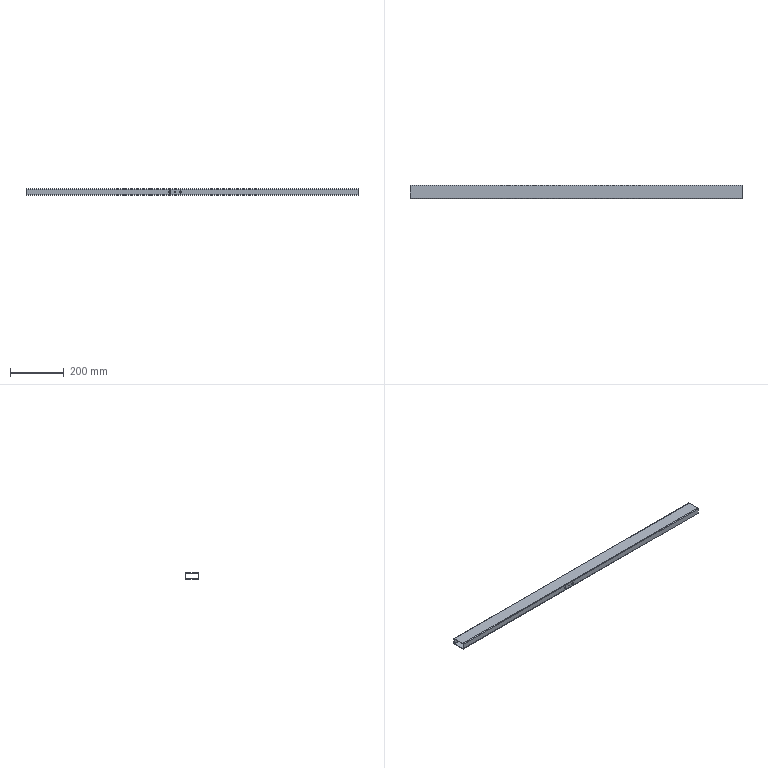Part | STEP file | 6150510 | 1 solid | 21 faces | box 1235 x 50 x 25 mm | volume 262357 mm3 | cylinder 11 | plane 10 | commonest cylinder face diameters 3 x4 5 x4 8 x2 3.2 x1
STEP:
#1=CARTESIAN_POINT('',(-617.5,-23.5,9.5));
#2=VERTEX_POINT('',#1);
#3=CARTESIAN_POINT('',(-617.5,-23.5,-9.5));
#4=VERTEX_POINT('',#3);
#5=CARTESIAN_POINT('',(-617.5,-23.5,9.5));
#6=DIRECTION('',(0.,0.,-1.));
#7=VECTOR('',#6,1000.);
#8=LINE('',#5,#7);
#9=EDGE_CURVE('',#2,#4,#8,.T.);
#10=ORIENTED_EDGE('',*,*,#9,.T.);
#11=CARTESIAN_POINT('',(-617.5,-22.,-11.));
#12=VERTEX_POINT('',#11);
#13=CARTESIAN_POINT('',(-617.5,-22.,-9.5));
#14=DIRECTION('',(1.,0.,0.));
#15=DIRECTION('',(0.,0.,-1.));
#16=AXIS2_PLACEMENT_3D('',#13,#14,#15);
#17=CIRCLE('',#16,1.5);
#18=EDGE_CURVE('',#4,#12,#17,.T.);
#19=ORIENTED_EDGE('',*,*,#18,.T.);
#20=CARTESIAN_POINT('',(-617.5,22.,-11.));
#21=VERTEX_POINT('',#20);
#22=CARTESIAN_POINT('',(-617.5,22.,-11.));
#23=DIRECTION('',(0.,1.,0.));
#24=VECTOR('',#23,1000.);
#25=LINE('',#22,#24);
#26=EDGE_CURVE('',#12,#21,#25,.T.);
#27=ORIENTED_EDGE('',*,*,#26,.T.);
#28=CARTESIAN_POINT('',(-617.5,23.5,-9.5));
#29=VERTEX_POINT('',#28);
#30=CARTESIAN_POINT('',(-617.5,22.,-9.5));
#31=DIRECTION('',(1.,0.,0.));
#32=DIRECTION('',(0.,0.,1.));
#33=AXIS2_PLACEMENT_3D('',#30,#31,#32);
#34=CIRCLE('',#33,1.5);
#35=EDGE_CURVE('',#21,#29,#34,.T.);
#36=ORIENTED_EDGE('',*,*,#35,.T.);
#37=CARTESIAN_POINT('',(-617.5,23.5,9.5));
#38=VERTEX_POINT('',#37);
#39=CARTESIAN_POINT('',(-617.5,23.5,9.5));
#40=DIRECTION('',(0.,0.,1.));
#41=VECTOR('',#40,1000.);
#42=LINE('',#39,#41);
#43=EDGE_CURVE('',#29,#38,#42,.T.);
#44=ORIENTED_EDGE('',*,*,#43,.T.);
#45=CARTESIAN_POINT('',(-617.5,22.,11.));
#46=VERTEX_POINT('',#45);
#47=CARTESIAN_POINT('',(-617.5,22.,9.5));
#48=DIRECTION('',(1.,0.,0.));
#49=DIRECTION('',(0.,0.,-1.));
#50=AXIS2_PLACEMENT_3D('',#47,#48,#49);
#51=CIRCLE('',#50,1.5);
#52=EDGE_CURVE('',#38,#46,#51,.T.);
#53=ORIENTED_EDGE('',*,*,#52,.T.);
#54=CARTESIAN_POINT('',(-617.5,-22.,11.));
#55=VERTEX_POINT('',#54);
#56=CARTESIAN_POINT('',(-617.5,22.,11.));
#57=DIRECTION('',(0.,-1.,0.));
#58=VECTOR('',#57,1000.);
#59=LINE('',#56,#58);
#60=EDGE_CURVE('',#46,#55,#59,.T.);
#61=ORIENTED_EDGE('',*,*,#60,.T.);
#62=CARTESIAN_POINT('',(-617.5,-22.,9.5));
#63=DIRECTION('',(1.,0.,0.));
#64=DIRECTION('',(0.,0.,-1.));
#65=AXIS2_PLACEMENT_3D('',#62,#63,#64);
#66=CIRCLE('',#65,1.5);
#67=EDGE_CURVE('',#55,#2,#66,.T.);
#68=ORIENTED_EDGE('',*,*,#67,.T.);
#69=EDGE_LOOP('',(#10,#19,#27,#36,#44,#53,#61,#68));
#70=FACE_BOUND('',#69,.T.);
#71=CARTESIAN_POINT('',(-617.5,-25.,10.));
#72=VERTEX_POINT('',#71);
#73=CARTESIAN_POINT('',(-617.5,-25.,-10.));
#74=VERTEX_POINT('',#73);
#75=CARTESIAN_POINT('',(-617.5,-25.,12.5));
#76=DIRECTION('',(0.,0.,-1.));
#77=VECTOR('',#76,1000.);
#78=LINE('',#75,#77);
#79=EDGE_CURVE('',#72,#74,#78,.T.);
#80=ORIENTED_EDGE('',*,*,#79,.F.);
#81=CARTESIAN_POINT('',(-617.5,-22.5,12.5));
#82=VERTEX_POINT('',#81);
#83=CARTESIAN_POINT('',(-617.5,-22.5,10.));
#84=DIRECTION('',(-1.,0.,0.));
#85=DIRECTION('',(0.,0.,-1.));
#86=AXIS2_PLACEMENT_3D('',#83,#84,#85);
#87=CIRCLE('',#86,2.5);
#88=EDGE_CURVE('',#72,#82,#87,.T.);
#89=ORIENTED_EDGE('',*,*,#88,.T.);
#90=CARTESIAN_POINT('',(-617.5,22.5,12.5));
#91=VERTEX_POINT('',#90);
#92=CARTESIAN_POINT('',(-617.5,25.,12.5));
#93=DIRECTION('',(0.,-1.,0.));
#94=VECTOR('',#93,1000.);
#95=LINE('',#92,#94);
#96=EDGE_CURVE('',#91,#82,#95,.T.);
#97=ORIENTED_EDGE('',*,*,#96,.F.);
#98=CARTESIAN_POINT('',(-617.5,25.,10.));
#99=VERTEX_POINT('',#98);
#100=CARTESIAN_POINT('',(-617.5,22.5,10.));
#101=DIRECTION('',(-1.,0.,0.));
#102=DIRECTION('',(0.,0.,-1.));
#103=AXIS2_PLACEMENT_3D('',#100,#101,#102);
#104=CIRCLE('',#103,2.5);
#105=EDGE_CURVE('',#91,#99,#104,.T.);
#106=ORIENTED_EDGE('',*,*,#105,.T.);
#107=CARTESIAN_POINT('',(-617.5,25.,-10.));
#108=VERTEX_POINT('',#107);
#109=CARTESIAN_POINT('',(-617.5,25.,12.5));
#110=DIRECTION('',(0.,0.,-1.));
#111=VECTOR('',#110,1000.);
#112=LINE('',#109,#111);
#113=EDGE_CURVE('',#99,#108,#112,.T.);
#114=ORIENTED_EDGE('',*,*,#113,.T.);
#115=CARTESIAN_POINT('',(-617.5,22.5,-12.5));
#116=VERTEX_POINT('',#115);
#117=CARTESIAN_POINT('',(-617.5,22.5,-10.));
#118=DIRECTION('',(-1.,0.,0.));
#119=DIRECTION('',(0.,0.,-1.));
#120=AXIS2_PLACEMENT_3D('',#117,#118,#119);
#121=CIRCLE('',#120,2.5);
#122=EDGE_CURVE('',#108,#116,#121,.T.);
#123=ORIENTED_EDGE('',*,*,#122,.T.);
#124=CARTESIAN_POINT('',(-617.5,-22.5,-12.5));
#125=VERTEX_POINT('',#124);
#126=CARTESIAN_POINT('',(-617.5,25.,-12.5));
#127=DIRECTION('',(0.,-1.,0.));
#128=VECTOR('',#127,1000.);
#129=LINE('',#126,#128);
#130=EDGE_CURVE('',#116,#125,#129,.T.);
#131=ORIENTED_EDGE('',*,*,#130,.T.);
#132=CARTESIAN_POINT('',(-617.5,-22.5,-10.));
#133=DIRECTION('',(-1.,0.,0.));
#134=DIRECTION('',(0.,0.,-1.));
#135=AXIS2_PLACEMENT_3D('',#132,#133,#134);
#136=CIRCLE('',#135,2.5);
#137=EDGE_CURVE('',#125,#74,#136,.T.);
#138=ORIENTED_EDGE('',*,*,#137,.T.);
#139=EDGE_LOOP('',(#80,#89,#97,#106,#114,#123,#131,#138));
#140=FACE_OUTER_BOUND('',#139,.T.);
#141=CARTESIAN_POINT('',(-617.5,25.,12.5));
#142=DIRECTION('',(1.,0.,0.));
#143=DIRECTION('',(0.,0.,-1.));
#144=AXIS2_PLACEMENT_3D('',#141,#142,#143);
#145=PLANE('',#144);
#146=ADVANCED_FACE('',(#70,#140),#145,.F.);
#147=CARTESIAN_POINT('',(-78.5,-25.,0.));
#148=VERTEX_POINT('',#147);
#149=CARTESIAN_POINT('',(-82.5,-25.,0.));
#150=DIRECTION('',(0.,-1.,0.));
#151=DIRECTION('',(1.,0.,0.));
#152=AXIS2_PLACEMENT_3D('',#149,#150,#151);
#153=CIRCLE('',#152,4.);
#154=EDGE_CURVE('',#148,#148,#153,.T.);
#155=ORIENTED_EDGE('',*,*,#154,.F.);
#156=EDGE_LOOP('',(#155));
#157=FACE_BOUND('',#156,.T.);
#158=CARTESIAN_POINT('',(-38.5,-25.,0.));
#159=VERTEX_POINT('',#158);
#160=CARTESIAN_POINT('',(-42.5,-25.,0.));
#161=DIRECTION('',(0.,-1.,0.));
#162=DIRECTION('',(1.,0.,0.));
#163=AXIS2_PLACEMENT_3D('',#160,#161,#162);
#164=CIRCLE('',#163,4.);
#165=EDGE_CURVE('',#159,#159,#164,.T.);
#166=ORIENTED_EDGE('',*,*,#165,.F.);
#167=EDGE_LOOP('',(#166));
#168=FACE_BOUND('',#167,.T.);
#169=CARTESIAN_POINT('',(-60.9,-25.,0.));
#170=VERTEX_POINT('',#169);
#171=CARTESIAN_POINT('',(-62.5,-25.,0.));
#172=DIRECTION('',(0.,-1.,0.));
#173=DIRECTION('',(1.,0.,0.));
#174=AXIS2_PLACEMENT_3D('',#171,#172,#173);
#175=CIRCLE('',#174,1.6);
#176=EDGE_CURVE('',#170,#170,#175,.T.);
#177=ORIENTED_EDGE('',*,*,#176,.F.);
#178=EDGE_LOOP('',(#177));
#179=FACE_BOUND('',#178,.T.);
#180=CARTESIAN_POINT('',(617.5,-25.,10.));
#181=VERTEX_POINT('',#180);
#182=CARTESIAN_POINT('',(617.5,-25.,-10.));
#183=VERTEX_POINT('',#182);
#184=CARTESIAN_POINT('',(617.5,-25.,12.5));
#185=DIRECTION('',(0.,0.,-1.));
#186=VECTOR('',#185,1000.);
#187=LINE('',#184,#186);
#188=EDGE_CURVE('',#181,#183,#187,.T.);
#189=ORIENTED_EDGE('',*,*,#188,.F.);
#190=CARTESIAN_POINT('',(-617.5,-25.,10.));
#191=DIRECTION('',(-1.,0.,0.));
#192=VECTOR('',#191,1000.);
#193=LINE('',#190,#192);
#194=EDGE_CURVE('',#181,#72,#193,.T.);
#195=ORIENTED_EDGE('',*,*,#194,.T.);
#196=ORIENTED_EDGE('',*,*,#79,.T.);
#197=CARTESIAN_POINT('',(-617.5,-25.,-10.));
#198=DIRECTION('',(1.,0.,0.));
#199=VECTOR('',#198,1000.);
#200=LINE('',#197,#199);
#201=EDGE_CURVE('',#74,#183,#200,.T.);
#202=ORIENTED_EDGE('',*,*,#201,.T.);
#203=EDGE_LOOP('',(#189,#195,#196,#202));
#204=FACE_OUTER_BOUND('',#203,.T.);
#205=CARTESIAN_POINT('',(-617.5,-25.,12.5));
#206=DIRECTION('',(0.,1.,0.));
#207=DIRECTION('',(-1.,0.,0.));
#208=AXIS2_PLACEMENT_3D('',#205,#206,#207);
#209=PLANE('',#208);
#210=ADVANCED_FACE('',(#157,#168,#179,#204),#209,.F.);
#211=CARTESIAN_POINT('',(617.5,-22.,-11.));
#212=VERTEX_POINT('',#211);
#213=CARTESIAN_POINT('',(617.5,22.,-11.));
#214=VERTEX_POINT('',#213);
#215=CARTESIAN_POINT('',(617.5,22.,-11.));
#216=DIRECTION('',(0.,1.,0.));
#217=VECTOR('',#216,1000.);
#218=LINE('',#215,#217);
#219=EDGE_CURVE('',#212,#214,#218,.T.);
#220=ORIENTED_EDGE('',*,*,#219,.F.);
#221=CARTESIAN_POINT('',(617.5,-23.5,-9.5));
#222=VERTEX_POINT('',#221);
#223=CARTESIAN_POINT('',(617.5,-22.,-9.5));
#224=DIRECTION('',(1.,0.,0.));
#225=DIRECTION('',(0.,0.,-1.));
#226=AXIS2_PLACEMENT_3D('',#223,#224,#225);
#227=CIRCLE('',#226,1.5);
#228=EDGE_CURVE('',#222,#212,#227,.T.);
#229=ORIENTED_EDGE('',*,*,#228,.F.);
#230=CARTESIAN_POINT('',(617.5,-23.5,9.5));
#231=VERTEX_POINT('',#230);
#232=CARTESIAN_POINT('',(617.5,-23.5,9.5));
#233=DIRECTION('',(0.,0.,-1.));
#234=VECTOR('',#233,1000.);
#235=LINE('',#232,#234);
#236=EDGE_CURVE('',#231,#222,#235,.T.);
#237=ORIENTED_EDGE('',*,*,#236,.F.);
#238=CARTESIAN_POINT('',(617.5,-22.,11.));
#239=VERTEX_POINT('',#238);
#240=CARTESIAN_POINT('',(617.5,-22.,9.5));
#241=DIRECTION('',(1.,0.,0.));
#242=DIRECTION('',(0.,0.,-1.));
#243=AXIS2_PLACEMENT_3D('',#240,#241,#242);
#244=CIRCLE('',#243,1.5);
#245=EDGE_CURVE('',#239,#231,#244,.T.);
#246=ORIENTED_EDGE('',*,*,#245,.F.);
#247=CARTESIAN_POINT('',(617.5,22.,11.));
#248=VERTEX_POINT('',#247);
#249=CARTESIAN_POINT('',(617.5,22.,11.));
#250=DIRECTION('',(0.,-1.,0.));
#251=VECTOR('',#250,1000.);
#252=LINE('',#249,#251);
#253=EDGE_CURVE('',#248,#239,#252,.T.);
#254=ORIENTED_EDGE('',*,*,#253,.F.);
#255=CARTESIAN_POINT('',(617.5,23.5,9.5));
#256=VERTEX_POINT('',#255);
#257=CARTESIAN_POINT('',(617.5,22.,9.5));
#258=DIRECTION('',(1.,0.,0.));
#259=DIRECTION('',(0.,0.,-1.));
#260=AXIS2_PLACEMENT_3D('',#257,#258,#259);
#261=CIRCLE('',#260,1.5);
#262=EDGE_CURVE('',#256,#248,#261,.T.);
#263=ORIENTED_EDGE('',*,*,#262,.F.);
#264=CARTESIAN_POINT('',(617.5,23.5,-9.5));
#265=VERTEX_POINT('',#264);
#266=CARTESIAN_POINT('',(617.5,23.5,9.5));
#267=DIRECTION('',(0.,0.,1.));
#268=VECTOR('',#267,1000.);
#269=LINE('',#266,#268);
#270=EDGE_CURVE('',#265,#256,#269,.T.);
#271=ORIENTED_EDGE('',*,*,#270,.F.);
#272=CARTESIAN_POINT('',(617.5,22.,-9.5));
#273=DIRECTION('',(1.,0.,0.));
#274=DIRECTION('',(0.,0.,1.));
#275=AXIS2_PLACEMENT_3D('',#272,#273,#274);
#276=CIRCLE('',#275,1.5);
#277=EDGE_CURVE('',#214,#265,#276,.T.);
#278=ORIENTED_EDGE('',*,*,#277,.F.);
#279=EDGE_LOOP('',(#220,#229,#237,#246,#254,#263,#271,#278));
#280=FACE_BOUND('',#279,.T.);
#281=CARTESIAN_POINT('',(617.5,-22.5,12.5));
#282=VERTEX_POINT('',#281);
#283=CARTESIAN_POINT('',(617.5,22.5,12.5));
#284=VERTEX_POINT('',#283);
#285=CARTESIAN_POINT('',(617.5,25.,12.5));
#286=DIRECTION('',(0.,1.,0.));
#287=VECTOR('',#286,1000.);
#288=LINE('',#285,#287);
#289=EDGE_CURVE('',#282,#284,#288,.T.);
#290=ORIENTED_EDGE('',*,*,#289,.F.);
#291=CARTESIAN_POINT('',(617.5,-22.5,10.));
#292=DIRECTION('',(1.,0.,0.));
#293=DIRECTION('',(0.,0.,1.));
#294=AXIS2_PLACEMENT_3D('',#291,#292,#293);
#295=CIRCLE('',#294,2.5);
#296=EDGE_CURVE('',#282,#181,#295,.T.);
#297=ORIENTED_EDGE('',*,*,#296,.T.);
#298=ORIENTED_EDGE('',*,*,#188,.T.);
#299=CARTESIAN_POINT('',(617.5,-22.5,-12.5));
#300=VERTEX_POINT('',#299);
#301=CARTESIAN_POINT('',(617.5,-22.5,-10.));
#302=DIRECTION('',(1.,0.,0.));
#303=DIRECTION('',(0.,0.,1.));
#304=AXIS2_PLACEMENT_3D('',#301,#302,#303);
#305=CIRCLE('',#304,2.5);
#306=EDGE_CURVE('',#183,#300,#305,.T.);
#307=ORIENTED_EDGE('',*,*,#306,.T.);
#308=CARTESIAN_POINT('',(617.5,22.5,-12.5));
#309=VERTEX_POINT('',#308);
#310=CARTESIAN_POINT('',(617.5,25.,-12.5));
#311=DIRECTION('',(0.,1.,0.));
#312=VECTOR('',#311,1000.);
#313=LINE('',#310,#312);
#314=EDGE_CURVE('',#300,#309,#313,.T.);
#315=ORIENTED_EDGE('',*,*,#314,.T.);
#316=CARTESIAN_POINT('',(617.5,25.,-10.));
#317=VERTEX_POINT('',#316);
#318=CARTESIAN_POINT('',(617.5,22.5,-10.));
#319=DIRECTION('',(1.,0.,0.));
#320=DIRECTION('',(0.,0.,1.));
#321=AXIS2_PLACEMENT_3D('',#318,#319,#320);
#322=CIRCLE('',#321,2.5);
#323=EDGE_CURVE('',#309,#317,#322,.T.);
#324=ORIENTED_EDGE('',*,*,#323,.T.);
#325=CARTESIAN_POINT('',(617.5,25.,10.));
#326=VERTEX_POINT('',#325);
#327=CARTESIAN_POINT('',(617.5,25.,12.5));
#328=DIRECTION('',(0.,0.,-1.));
#329=VECTOR('',#328,1000.);
#330=LINE('',#327,#329);
#331=EDGE_CURVE('',#326,#317,#330,.T.);
#332=ORIENTED_EDGE('',*,*,#331,.F.);
#333=CARTESIAN_POINT('',(617.5,22.5,10.));
#334=DIRECTION('',(1.,0.,0.));
#335=DIRECTION('',(0.,0.,1.));
#336=AXIS2_PLACEMENT_3D('',#333,#334,#335);
#337=CIRCLE('',#336,2.5);
#338=EDGE_CURVE('',#326,#284,#337,.T.);
#339=ORIENTED_EDGE('',*,*,#338,.T.);
#340=EDGE_LOOP('',(#290,#297,#298,#307,#315,#324,#332,#339));
#341=FACE_OUTER_BOUND('',#340,.T.);
#342=CARTESIAN_POINT('',(617.5,25.,12.5));
#343=DIRECTION('',(-1.,0.,0.));
#344=DIRECTION('',(0.,0.,1.));
#345=AXIS2_PLACEMENT_3D('',#342,#343,#344);
#346=PLANE('',#345);
#347=ADVANCED_FACE('',(#280,#341),#346,.F.);
#348=ORIENTED_EDGE('',*,*,#331,.T.);
#349=CARTESIAN_POINT('',(-617.5,25.,-10.));
#350=DIRECTION('',(-1.,0.,0.));
#351=VECTOR('',#350,1000.);
#352=LINE('',#349,#351);
#353=EDGE_CURVE('',#317,#108,#352,.T.);
#354=ORIENTED_EDGE('',*,*,#353,.T.);
#355=ORIENTED_EDGE('',*,*,#113,.F.);
#356=CARTESIAN_POINT('',(617.5,25.,10.));
#357=DIRECTION('',(1.,0.,0.));
#358=VECTOR('',#357,1000.);
#359=LINE('',#356,#358);
#360=EDGE_CURVE('',#99,#326,#359,.T.);
#361=ORIENTED_EDGE('',*,*,#360,.T.);
#362=EDGE_LOOP('',(#348,#354,#355,#361));
#363=FACE_OUTER_BOUND('',#362,.T.);
#364=CARTESIAN_POINT('',(-617.5,25.,12.5));
#365=DIRECTION('',(0.,-1.,0.));
#366=DIRECTION('',(0.,0.,-1.));
#367=AXIS2_PLACEMENT_3D('',#364,#365,#366);
#368=PLANE('',#367);
#369=ADVANCED_FACE('',(#363),#368,.F.);
#370=ORIENTED_EDGE('',*,*,#96,.T.);
#371=CARTESIAN_POINT('',(617.5,-22.5,12.5));
#372=DIRECTION('',(1.,0.,0.));
#373=VECTOR('',#372,1000.);
#374=LINE('',#371,#373);
#375=EDGE_CURVE('',#82,#282,#374,.T.);
#376=ORIENTED_EDGE('',*,*,#375,.T.);
#377=ORIENTED_EDGE('',*,*,#289,.T.);
#378=CARTESIAN_POINT('',(-617.5,22.5,12.5));
#379=DIRECTION('',(-1.,0.,0.));
#380=VECTOR('',#379,1000.);
#381=LINE('',#378,#380);
#382=EDGE_CURVE('',#284,#91,#381,.T.);
#383=ORIENTED_EDGE('',*,*,#382,.T.);
#384=EDGE_LOOP('',(#370,#376,#377,#383));
#385=FACE_OUTER_BOUND('',#384,.T.);
#386=CARTESIAN_POINT('',(-617.5,25.,12.5));
#387=DIRECTION('',(0.,0.,1.));
#388=DIRECTION('',(1.,0.,0.));
#389=AXIS2_PLACEMENT_3D('',#386,#387,#388);
#390=PLANE('',#389);
#391=ADVANCED_FACE('',(#385),#390,.T.);
#392=ORIENTED_EDGE('',*,*,#314,.F.);
#393=CARTESIAN_POINT('',(-617.5,-22.5,-12.5));
#394=DIRECTION('',(-1.,0.,0.));
#395=VECTOR('',#394,1000.);
#396=LINE('',#393,#395);
#397=EDGE_CURVE('',#300,#125,#396,.T.);
#398=ORIENTED_EDGE('',*,*,#397,.T.);
#399=ORIENTED_EDGE('',*,*,#130,.F.);
#400=CARTESIAN_POINT('',(-617.5,22.5,-12.5));
#401=DIRECTION('',(1.,0.,0.));
#402=VECTOR('',#401,1000.);
#403=LINE('',#400,#402);
#404=EDGE_CURVE('',#116,#309,#403,.T.);
#405=ORIENTED_EDGE('',*,*,#404,.T.);
#406=EDGE_LOOP('',(#392,#398,#399,#405));
#407=FACE_OUTER_BOUND('',#406,.T.);
#408=CARTESIAN_POINT('',(-617.5,25.,-12.5));
#409=DIRECTION('',(0.,0.,1.));
#410=DIRECTION('',(1.,0.,0.));
#411=AXIS2_PLACEMENT_3D('',#408,#409,#410);
#412=PLANE('',#411);
#413=ADVANCED_FACE('',(#407),#412,.F.);
#414=ORIENTED_EDGE('',*,*,#88,.F.);
#415=ORIENTED_EDGE('',*,*,#194,.F.);
#416=ORIENTED_EDGE('',*,*,#296,.F.);
#417=ORIENTED_EDGE('',*,*,#375,.F.);
#418=EDGE_LOOP('',(#414,#415,#416,#417));
#419=FACE_OUTER_BOUND('',#418,.T.);
#420=CARTESIAN_POINT('',(-617.5,-22.5,10.));
#421=DIRECTION('',(-1.,0.,0.));
#422=DIRECTION('',(0.,-1.,0.));
#423=AXIS2_PLACEMENT_3D('',#420,#421,#422);
#424=CYLINDRICAL_SURFACE('',#423,2.5);
#425=ADVANCED_FACE('',(#419),#424,.T.);
#426=ORIENTED_EDGE('',*,*,#137,.F.);
#427=ORIENTED_EDGE('',*,*,#397,.F.);
#428=ORIENTED_EDGE('',*,*,#306,.F.);
#429=ORIENTED_EDGE('',*,*,#201,.F.);
#430=EDGE_LOOP('',(#426,#427,#428,#429));
#431=FACE_OUTER_BOUND('',#430,.T.);
#432=CARTESIAN_POINT('',(-617.5,-22.5,-10.));
#433=DIRECTION('',(1.,0.,0.));
#434=DIRECTION('',(0.,1.,0.));
#435=AXIS2_PLACEMENT_3D('',#432,#433,#434);
#436=CYLINDRICAL_SURFACE('',#435,2.5);
#437=ADVANCED_FACE('',(#431),#436,.T.);
#438=ORIENTED_EDGE('',*,*,#323,.F.);
#439=ORIENTED_EDGE('',*,*,#404,.F.);
#440=ORIENTED_EDGE('',*,*,#122,.F.);
#441=ORIENTED_EDGE('',*,*,#353,.F.);
#442=EDGE_LOOP('',(#438,#439,#440,#441));
#443=FACE_OUTER_BOUND('',#442,.T.);
#444=CARTESIAN_POINT('',(-617.5,22.5,-10.));
#445=DIRECTION('',(-1.,0.,0.));
#446=DIRECTION('',(0.,0.,1.));
#447=AXIS2_PLACEMENT_3D('',#444,#445,#446);
#448=CYLINDRICAL_SURFACE('',#447,2.5);
#449=ADVANCED_FACE('',(#443),#448,.T.);
#450=ORIENTED_EDGE('',*,*,#338,.F.);
#451=ORIENTED_EDGE('',*,*,#360,.F.);
#452=ORIENTED_EDGE('',*,*,#105,.F.);
#453=ORIENTED_EDGE('',*,*,#382,.F.);
#454=EDGE_LOOP('',(#450,#451,#452,#453));
#455=FACE_OUTER_BOUND('',#454,.T.);
#456=CARTESIAN_POINT('',(-617.5,22.5,10.));
#457=DIRECTION('',(1.,0.,0.));
#458=DIRECTION('',(0.,0.,-1.));
#459=AXIS2_PLACEMENT_3D('',#456,#457,#458);
#460=CYLINDRICAL_SURFACE('',#459,2.5);
#461=ADVANCED_FACE('',(#455),#460,.T.);
#462=ORIENTED_EDGE('',*,*,#228,.T.);
#463=CARTESIAN_POINT('',(-617.5,-22.,-11.));
#464=DIRECTION('',(1.,0.,0.));
#465=VECTOR('',#464,1000.);
#466=LINE('',#463,#465);
#467=EDGE_CURVE('',#12,#212,#466,.T.);
#468=ORIENTED_EDGE('',*,*,#467,.F.);
#469=ORIENTED_EDGE('',*,*,#18,.F.);
#470=CARTESIAN_POINT('',(-617.5,-23.5,-9.5));
#471=DIRECTION('',(1.,0.,0.));
#472=VECTOR('',#471,1000.);
#473=LINE('',#470,#472);
#474=EDGE_CURVE('',#4,#222,#473,.T.);
#475=ORIENTED_EDGE('',*,*,#474,.T.);
#476=EDGE_LOOP('',(#462,#468,#469,#475));
#477=FACE_OUTER_BOUND('',#476,.T.);
#478=CARTESIAN_POINT('',(-617.5,-22.,-9.5));
#479=DIRECTION('',(1.,0.,0.));
#480=DIRECTION('',(0.,0.,-1.));
#481=AXIS2_PLACEMENT_3D('',#478,#479,#480);
#482=CYLINDRICAL_SURFACE('',#481,1.5);
#483=ADVANCED_FACE('',(#477),#482,.F.);
#484=CARTESIAN_POINT('',(-82.5,-23.5,-4.));
#485=VERTEX_POINT('',#484);
#486=CARTESIAN_POINT('',(-82.5,-23.5,0.));
#487=DIRECTION('',(0.,-1.,0.));
#488=DIRECTION('',(0.,0.,-1.));
#489=AXIS2_PLACEMENT_3D('',#486,#487,#488);
#490=CIRCLE('',#489,4.);
#491=EDGE_CURVE('',#485,#485,#490,.T.);
#492=ORIENTED_EDGE('',*,*,#491,.T.);
#493=EDGE_LOOP('',(#492));
#494=FACE_BOUND('',#493,.T.);
#495=CARTESIAN_POINT('',(-42.5,-23.5,-4.));
#496=VERTEX_POINT('',#495);
#497=CARTESIAN_POINT('',(-42.5,-23.5,0.));
#498=DIRECTION('',(0.,-1.,0.));
#499=DIRECTION('',(0.,0.,-1.));
#500=AXIS2_PLACEMENT_3D('',#497,#498,#499);
#501=CIRCLE('',#500,4.);
#502=EDGE_CURVE('',#496,#496,#501,.T.);
#503=ORIENTED_EDGE('',*,*,#502,.T.);
#504=EDGE_LOOP('',(#503));
#505=FACE_BOUND('',#504,.T.);
#506=CARTESIAN_POINT('',(-62.5,-23.5,-1.6));
#507=VERTEX_POINT('',#506);
#508=CARTESIAN_POINT('',(-62.5,-23.5,0.));
#509=DIRECTION('',(0.,-1.,0.));
#510=DIRECTION('',(0.,0.,-1.));
#511=AXIS2_PLACEMENT_3D('',#508,#509,#510);
#512=CIRCLE('',#511,1.6);
#513=EDGE_CURVE('',#507,#507,#512,.T.);
#514=ORIENTED_EDGE('',*,*,#513,.T.);
#515=EDGE_LOOP('',(#514));
#516=FACE_BOUND('',#515,.T.);
#517=ORIENTED_EDGE('',*,*,#236,.T.);
#518=ORIENTED_EDGE('',*,*,#474,.F.);
#519=ORIENTED_EDGE('',*,*,#9,.F.);
#520=CARTESIAN_POINT('',(-617.5,-23.5,9.5));
#521=DIRECTION('',(1.,0.,0.));
#522=VECTOR('',#521,1000.);
#523=LINE('',#520,#522);
#524=EDGE_CURVE('',#2,#231,#523,.T.);
#525=ORIENTED_EDGE('',*,*,#524,.T.);
#526=EDGE_LOOP('',(#517,#518,#519,#525));
#527=FACE_OUTER_BOUND('',#526,.T.);
#528=CARTESIAN_POINT('',(-617.5,-23.5,9.5));
#529=DIRECTION('',(0.,-1.,0.));
#530=DIRECTION('',(0.,0.,-1.));
#531=AXIS2_PLACEMENT_3D('',#528,#529,#530);
#532=PLANE('',#531);
#533=ADVANCED_FACE('',(#494,#505,#516,#527),#532,.F.);
#534=ORIENTED_EDGE('',*,*,#245,.T.);
#535=ORIENTED_EDGE('',*,*,#524,.F.);
#536=ORIENTED_EDGE('',*,*,#67,.F.);
#537=CARTESIAN_POINT('',(-617.5,-22.,11.));
#538=DIRECTION('',(1.,0.,0.));
#539=VECTOR('',#538,1000.);
#540=LINE('',#537,#539);
#541=EDGE_CURVE('',#55,#239,#540,.T.);
#542=ORIENTED_EDGE('',*,*,#541,.T.);
#543=EDGE_LOOP('',(#534,#535,#536,#542));
#544=FACE_OUTER_BOUND('',#543,.T.);
#545=CARTESIAN_POINT('',(-617.5,-22.,9.5));
#546=DIRECTION('',(1.,0.,0.));
#547=DIRECTION('',(0.,0.,-1.));
#548=AXIS2_PLACEMENT_3D('',#545,#546,#547);
#549=CYLINDRICAL_SURFACE('',#548,1.5);
#550=ADVANCED_FACE('',(#544),#549,.F.);
#551=ORIENTED_EDGE('',*,*,#253,.T.);
#552=ORIENTED_EDGE('',*,*,#541,.F.);
#553=ORIENTED_EDGE('',*,*,#60,.F.);
#554=CARTESIAN_POINT('',(-617.5,22.,11.));
#555=DIRECTION('',(1.,0.,0.));
#556=VECTOR('',#555,1000.);
#557=LINE('',#554,#556);
#558=EDGE_CURVE('',#46,#248,#557,.T.);
#559=ORIENTED_EDGE('',*,*,#558,.T.);
#560=EDGE_LOOP('',(#551,#552,#553,#559));
#561=FACE_OUTER_BOUND('',#560,.T.);
#562=CARTESIAN_POINT('',(-617.5,22.,11.));
#563=DIRECTION('',(0.,0.,1.));
#564=DIRECTION('',(0.,-1.,0.));
#565=AXIS2_PLACEMENT_3D('',#562,#563,#564);
#566=PLANE('',#565);
#567=ADVANCED_FACE('',(#561),#566,.F.);
#568=ORIENTED_EDGE('',*,*,#262,.T.);
#569=ORIENTED_EDGE('',*,*,#558,.F.);
#570=ORIENTED_EDGE('',*,*,#52,.F.);
#571=CARTESIAN_POINT('',(-617.5,23.5,9.5));
#572=DIRECTION('',(1.,0.,0.));
#573=VECTOR('',#572,1000.);
#574=LINE('',#571,#573);
#575=EDGE_CURVE('',#38,#256,#574,.T.);
#576=ORIENTED_EDGE('',*,*,#575,.T.);
#577=EDGE_LOOP('',(#568,#569,#570,#576));
#578=FACE_OUTER_BOUND('',#577,.T.);
#579=CARTESIAN_POINT('',(-617.5,22.,9.5));
#580=DIRECTION('',(1.,0.,0.));
#581=DIRECTION('',(0.,0.,-1.));
#582=AXIS2_PLACEMENT_3D('',#579,#580,#581);
#583=CYLINDRICAL_SURFACE('',#582,1.5);
#584=ADVANCED_FACE('',(#578),#583,.F.);
#585=ORIENTED_EDGE('',*,*,#270,.T.);
#586=ORIENTED_EDGE('',*,*,#575,.F.);
#587=ORIENTED_EDGE('',*,*,#43,.F.);
#588=CARTESIAN_POINT('',(-617.5,23.5,-9.5));
#589=DIRECTION('',(1.,0.,0.));
#590=VECTOR('',#589,1000.);
#591=LINE('',#588,#590);
#592=EDGE_CURVE('',#29,#265,#591,.T.);
#593=ORIENTED_EDGE('',*,*,#592,.T.);
#594=EDGE_LOOP('',(#585,#586,#587,#593));
#595=FACE_OUTER_BOUND('',#594,.T.);
#596=CARTESIAN_POINT('',(-617.5,23.5,9.5));
#597=DIRECTION('',(0.,1.,0.));
#598=DIRECTION('',(0.,0.,1.));
#599=AXIS2_PLACEMENT_3D('',#596,#597,#598);
#600=PLANE('',#599);
#601=ADVANCED_FACE('',(#595),#600,.F.);
#602=ORIENTED_EDGE('',*,*,#277,.T.);
#603=ORIENTED_EDGE('',*,*,#592,.F.);
#604=ORIENTED_EDGE('',*,*,#35,.F.);
#605=CARTESIAN_POINT('',(-617.5,22.,-11.));
#606=DIRECTION('',(1.,0.,0.));
#607=VECTOR('',#606,1000.);
#608=LINE('',#605,#607);
#609=EDGE_CURVE('',#21,#214,#608,.T.);
#610=ORIENTED_EDGE('',*,*,#609,.T.);
#611=EDGE_LOOP('',(#602,#603,#604,#610));
#612=FACE_OUTER_BOUND('',#611,.T.);
#613=CARTESIAN_POINT('',(-617.5,22.,-9.5));
#614=DIRECTION('',(1.,0.,0.));
#615=DIRECTION('',(0.,0.,-1.));
#616=AXIS2_PLACEMENT_3D('',#613,#614,#615);
#617=CYLINDRICAL_SURFACE('',#616,1.5);
#618=ADVANCED_FACE('',(#612),#617,.F.);
#619=ORIENTED_EDGE('',*,*,#219,.T.);
#620=ORIENTED_EDGE('',*,*,#609,.F.);
#621=ORIENTED_EDGE('',*,*,#26,.F.);
#622=ORIENTED_EDGE('',*,*,#467,.T.);
#623=EDGE_LOOP('',(#619,#620,#621,#622));
#624=FACE_OUTER_BOUND('',#623,.T.);
#625=CARTESIAN_POINT('',(-617.5,22.,-11.));
#626=DIRECTION('',(0.,0.,-1.));
#627=DIRECTION('',(0.,1.,0.));
#628=AXIS2_PLACEMENT_3D('',#625,#626,#627);
#629=PLANE('',#628);
#630=ADVANCED_FACE('',(#624),#629,.F.);
#631=ORIENTED_EDGE('',*,*,#176,.T.);
#632=EDGE_LOOP('',(#631));
#633=FACE_OUTER_BOUND('',#632,.T.);
#634=ORIENTED_EDGE('',*,*,#513,.F.);
#635=EDGE_LOOP('',(#634));
#636=FACE_OUTER_BOUND('',#635,.T.);
#637=CARTESIAN_POINT('',(-62.5,-15.,0.));
#638=DIRECTION('',(0.,-1.,0.));
#639=DIRECTION('',(1.,0.,0.));
#640=AXIS2_PLACEMENT_3D('',#637,#638,#639);
#641=CYLINDRICAL_SURFACE('',#640,1.6);
#642=ADVANCED_FACE('',(#633,#636),#641,.F.);
#643=ORIENTED_EDGE('',*,*,#165,.T.);
#644=EDGE_LOOP('',(#643));
#645=FACE_OUTER_BOUND('',#644,.T.);
#646=ORIENTED_EDGE('',*,*,#502,.F.);
#647=EDGE_LOOP('',(#646));
#648=FACE_OUTER_BOUND('',#647,.T.);
#649=CARTESIAN_POINT('',(-42.5,-15.,0.));
#650=DIRECTION('',(0.,-1.,0.));
#651=DIRECTION('',(1.,0.,0.));
#652=AXIS2_PLACEMENT_3D('',#649,#650,#651);
#653=CYLINDRICAL_SURFACE('',#652,4.);
#654=ADVANCED_FACE('',(#645,#648),#653,.F.);
#655=ORIENTED_EDGE('',*,*,#154,.T.);
#656=EDGE_LOOP('',(#655));
#657=FACE_OUTER_BOUND('',#656,.T.);
#658=ORIENTED_EDGE('',*,*,#491,.F.);
#659=EDGE_LOOP('',(#658));
#660=FACE_OUTER_BOUND('',#659,.T.);
#661=CARTESIAN_POINT('',(-82.5,-15.,0.));
#662=DIRECTION('',(0.,-1.,0.));
#663=DIRECTION('',(1.,0.,0.));
#664=AXIS2_PLACEMENT_3D('',#661,#662,#663);
#665=CYLINDRICAL_SURFACE('',#664,4.);
#666=ADVANCED_FACE('',(#657,#660),#665,.F.);
#667=CLOSED_SHELL('',(#146,#210,#347,#369,#391,#413,#425,#437,#449,#461,#483,#533,#550,#567,#584,#601,#618,#630,#642,#654,#666));
#668=MANIFOLD_SOLID_BREP('',#667);
#669=CARTESIAN_POINT('',(0.,0.,0.));
#670=DIRECTION('',(0.,0.,1.));
#671=DIRECTION('',(1.,0.,0.));
#672=AXIS2_PLACEMENT_3D('',#669,#670,#671);
#673=(LENGTH_UNIT()NAMED_UNIT(*)SI_UNIT(.MILLI.,.METRE.));
#674=UNCERTAINTY_MEASURE_WITH_UNIT(LENGTH_MEASURE(0.00001),#673,'','');
#675=(NAMED_UNIT(*)PLANE_ANGLE_UNIT()SI_UNIT($,.RADIAN.));
#676=(NAMED_UNIT(*)SI_UNIT($,.STERADIAN.)SOLID_ANGLE_UNIT());
#677=(GEOMETRIC_REPRESENTATION_CONTEXT(3)GLOBAL_UNCERTAINTY_ASSIGNED_CONTEXT((#674))GLOBAL_UNIT_ASSIGNED_CONTEXT((#673,#675,#676))REPRESENTATION_CONTEXT('',''));
#678=ADVANCED_BREP_SHAPE_REPRESENTATION('',(#668,#672),#677);